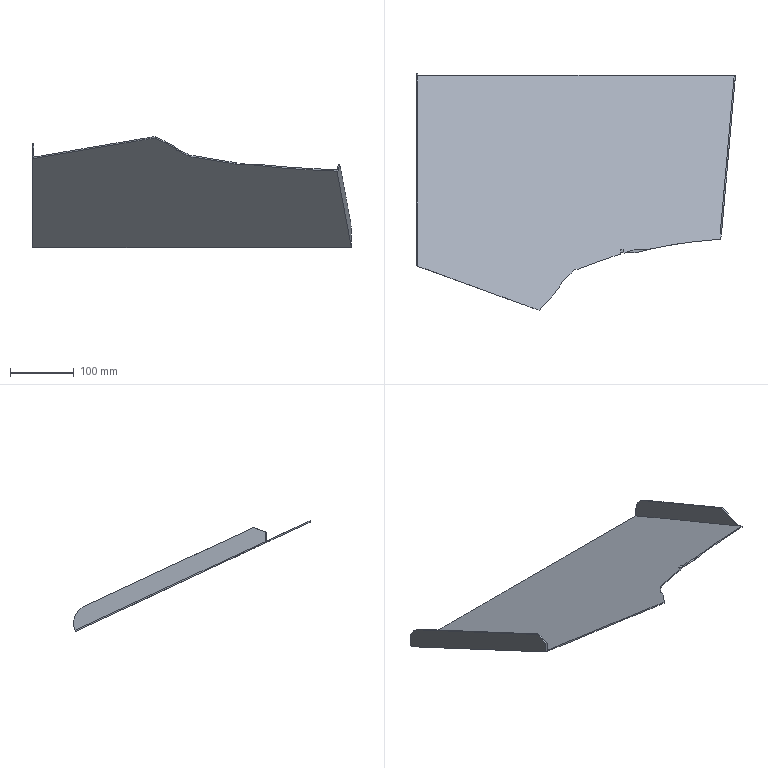Part | NX | features solid 2 | 1 solid | 21 faces | box 501.81 x 372.646 x 174.664 mm | volume 353855 mm3 | plane 12 | spline 7 | cylinder 2 | commonest cylinder face diameters 60 x2